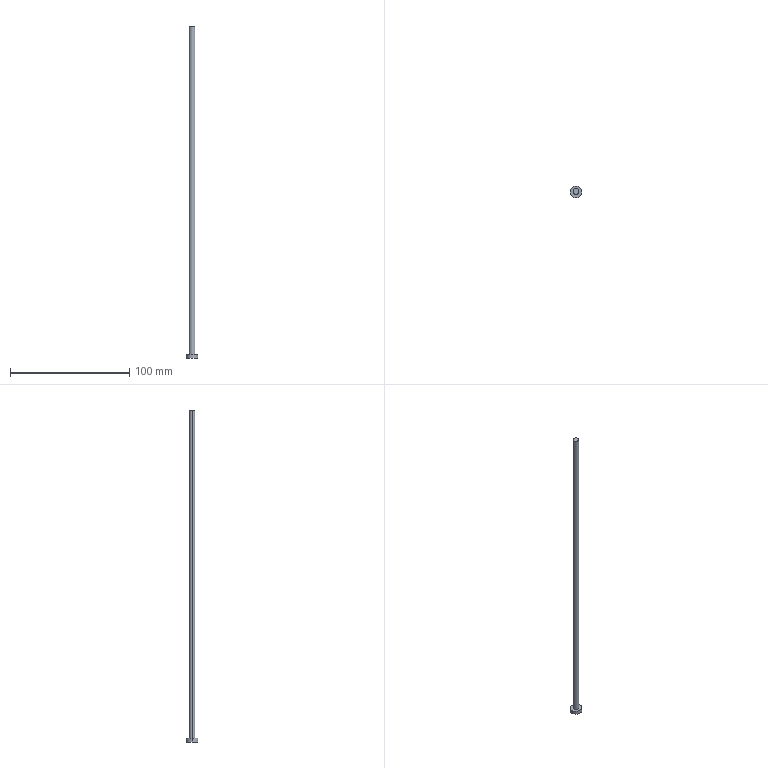Part | Creo | 1 solid | 7 faces | box 10 x 10 x 278.48 mm | volume 5645 mm3 | cylinder 4 | plane 3 | commonest cylinder face diameters 5 x2 10 x2
STEP:
#1=CARTESIAN_POINT('',(-182.5,235.,42.98));
#2=VERTEX_POINT('',#1);
#3=CARTESIAN_POINT('',(-187.5,235.,42.98));
#4=VERTEX_POINT('',#3);
#5=CARTESIAN_POINT('',(-185.,235.,42.98));
#6=DIRECTION('',(0.,0.,1.));
#7=DIRECTION('',(1.,0.,0.));
#8=AXIS2_PLACEMENT_3D('',#5,#6,#7);
#9=CIRCLE('',#8,2.5);
#10=EDGE_CURVE('',#2,#4,#9,.T.);
#11=ORIENTED_EDGE('',*,*,#10,.T.);
#12=CARTESIAN_POINT('',(-187.5,235.,-232.5));
#13=VERTEX_POINT('',#12);
#14=CARTESIAN_POINT('',(-187.5,235.,42.98));
#15=DIRECTION('',(0.,0.,-1.));
#16=VECTOR('',#15,275.48);
#17=LINE('',#14,#16);
#18=EDGE_CURVE('',#4,#13,#17,.T.);
#19=ORIENTED_EDGE('',*,*,#18,.T.);
#20=CARTESIAN_POINT('',(-182.5,235.,-232.5));
#21=VERTEX_POINT('',#20);
#22=CARTESIAN_POINT('',(-185.,235.,-232.5));
#23=DIRECTION('',(0.,0.,-1.));
#24=DIRECTION('',(-1.,0.,0.));
#25=AXIS2_PLACEMENT_3D('',#22,#23,#24);
#26=CIRCLE('',#25,2.5);
#27=EDGE_CURVE('',#13,#21,#26,.T.);
#28=ORIENTED_EDGE('',*,*,#27,.T.);
#29=CARTESIAN_POINT('',(-182.5,235.,42.98));
#30=DIRECTION('',(0.,0.,-1.));
#31=VECTOR('',#30,275.48);
#32=LINE('',#29,#31);
#33=EDGE_CURVE('',#2,#21,#32,.T.);
#34=ORIENTED_EDGE('',*,*,#33,.F.);
#35=EDGE_LOOP('',(#11,#19,#28,#34));
#36=FACE_OUTER_BOUND('',#35,.F.);
#37=CARTESIAN_POINT('',(-185.,235.,49.5));
#38=DIRECTION('',(0.,0.,-1.));
#39=DIRECTION('',(-1.,0.,0.));
#40=AXIS2_PLACEMENT_3D('',#37,#38,#39);
#41=CYLINDRICAL_SURFACE('',#40,2.5);
#42=ADVANCED_FACE('',(#36),#41,.T.);
#43=CARTESIAN_POINT('',(-185.,235.,42.98));
#44=DIRECTION('',(0.,0.,1.));
#45=DIRECTION('',(-1.,0.,0.));
#46=AXIS2_PLACEMENT_3D('',#43,#44,#45);
#47=CIRCLE('',#46,2.5);
#48=EDGE_CURVE('',#4,#2,#47,.T.);
#49=ORIENTED_EDGE('',*,*,#48,.F.);
#50=ORIENTED_EDGE('',*,*,#10,.F.);
#51=EDGE_LOOP('',(#49,#50));
#52=FACE_OUTER_BOUND('',#51,.F.);
#53=CARTESIAN_POINT('',(-179.214,-235.438,42.98));
#54=DIRECTION('',(0.,0.,-1.));
#55=DIRECTION('',(0.,1.,0.));
#56=AXIS2_PLACEMENT_3D('',#53,#54,#55);
#57=PLANE('',#56);
#58=ADVANCED_FACE('',(#52),#57,.F.);
#59=ORIENTED_EDGE('',*,*,#48,.T.);
#60=ORIENTED_EDGE('',*,*,#33,.T.);
#61=CARTESIAN_POINT('',(-185.,235.,-232.5));
#62=DIRECTION('',(0.,0.,-1.));
#63=DIRECTION('',(1.,0.,0.));
#64=AXIS2_PLACEMENT_3D('',#61,#62,#63);
#65=CIRCLE('',#64,2.5);
#66=EDGE_CURVE('',#21,#13,#65,.T.);
#67=ORIENTED_EDGE('',*,*,#66,.T.);
#68=ORIENTED_EDGE('',*,*,#18,.F.);
#69=EDGE_LOOP('',(#59,#60,#67,#68));
#70=FACE_OUTER_BOUND('',#69,.F.);
#71=CARTESIAN_POINT('',(-185.,235.,49.5));
#72=DIRECTION('',(0.,0.,-1.));
#73=DIRECTION('',(-1.,0.,0.));
#74=AXIS2_PLACEMENT_3D('',#71,#72,#73);
#75=CYLINDRICAL_SURFACE('',#74,2.5);
#76=ADVANCED_FACE('',(#70),#75,.T.);
#77=CARTESIAN_POINT('',(-190.,235.,-232.5));
#78=VERTEX_POINT('',#77);
#79=CARTESIAN_POINT('',(-180.,235.,-232.5));
#80=VERTEX_POINT('',#79);
#81=CARTESIAN_POINT('',(-185.,235.,-232.5));
#82=DIRECTION('',(0.,0.,1.));
#83=DIRECTION('',(-1.,0.,0.));
#84=AXIS2_PLACEMENT_3D('',#81,#82,#83);
#85=CIRCLE('',#84,5.);
#86=EDGE_CURVE('',#78,#80,#85,.T.);
#87=ORIENTED_EDGE('',*,*,#86,.F.);
#88=CARTESIAN_POINT('',(-185.,235.,-232.5));
#89=DIRECTION('',(0.,0.,1.));
#90=DIRECTION('',(1.,0.,0.));
#91=AXIS2_PLACEMENT_3D('',#88,#89,#90);
#92=CIRCLE('',#91,5.);
#93=EDGE_CURVE('',#80,#78,#92,.T.);
#94=ORIENTED_EDGE('',*,*,#93,.F.);
#95=EDGE_LOOP('',(#87,#94));
#96=FACE_OUTER_BOUND('',#95,.F.);
#97=ORIENTED_EDGE('',*,*,#27,.F.);
#98=ORIENTED_EDGE('',*,*,#66,.F.);
#99=EDGE_LOOP('',(#97,#98));
#100=FACE_BOUND('',#99,.F.);
#101=CARTESIAN_POINT('',(-185.,235.,-232.5));
#102=DIRECTION('',(0.,0.,-1.));
#103=DIRECTION('',(-1.,0.,0.));
#104=AXIS2_PLACEMENT_3D('',#101,#102,#103);
#105=PLANE('',#104);
#106=ADVANCED_FACE('',(#96,#100),#105,.F.);
#107=CARTESIAN_POINT('',(-180.,235.,-235.5));
#108=VERTEX_POINT('',#107);
#109=CARTESIAN_POINT('',(-190.,235.,-235.5));
#110=VERTEX_POINT('',#109);
#111=CARTESIAN_POINT('',(-185.,235.,-235.5));
#112=DIRECTION('',(0.,0.,-1.));
#113=DIRECTION('',(1.,0.,0.));
#114=AXIS2_PLACEMENT_3D('',#111,#112,#113);
#115=CIRCLE('',#114,5.);
#116=EDGE_CURVE('',#108,#110,#115,.T.);
#117=ORIENTED_EDGE('',*,*,#116,.T.);
#118=CARTESIAN_POINT('',(-190.,235.,-232.5));
#119=DIRECTION('',(0.,0.,-1.));
#120=VECTOR('',#119,3.);
#121=LINE('',#118,#120);
#122=EDGE_CURVE('',#78,#110,#121,.T.);
#123=ORIENTED_EDGE('',*,*,#122,.F.);
#124=ORIENTED_EDGE('',*,*,#86,.T.);
#125=CARTESIAN_POINT('',(-180.,235.,-232.5));
#126=DIRECTION('',(0.,0.,-1.));
#127=VECTOR('',#126,3.);
#128=LINE('',#125,#127);
#129=EDGE_CURVE('',#80,#108,#128,.T.);
#130=ORIENTED_EDGE('',*,*,#129,.T.);
#131=EDGE_LOOP('',(#117,#123,#124,#130));
#132=FACE_OUTER_BOUND('',#131,.F.);
#133=CARTESIAN_POINT('',(-185.,235.,-245.913));
#134=DIRECTION('',(0.,0.,-1.));
#135=DIRECTION('',(-1.,0.,0.));
#136=AXIS2_PLACEMENT_3D('',#133,#134,#135);
#137=CYLINDRICAL_SURFACE('',#136,5.);
#138=ADVANCED_FACE('',(#132),#137,.T.);
#139=ORIENTED_EDGE('',*,*,#116,.F.);
#140=CARTESIAN_POINT('',(-185.,235.,-235.5));
#141=DIRECTION('',(0.,0.,-1.));
#142=DIRECTION('',(-1.,0.,0.));
#143=AXIS2_PLACEMENT_3D('',#140,#141,#142);
#144=CIRCLE('',#143,5.);
#145=EDGE_CURVE('',#110,#108,#144,.T.);
#146=ORIENTED_EDGE('',*,*,#145,.F.);
#147=EDGE_LOOP('',(#139,#146));
#148=FACE_OUTER_BOUND('',#147,.F.);
#149=CARTESIAN_POINT('',(-181.,235.,-235.5));
#150=DIRECTION('',(0.,0.,1.));
#151=DIRECTION('',(1.,0.,0.));
#152=AXIS2_PLACEMENT_3D('',#149,#150,#151);
#153=PLANE('',#152);
#154=ADVANCED_FACE('',(#148),#153,.F.);
#155=ORIENTED_EDGE('',*,*,#145,.T.);
#156=ORIENTED_EDGE('',*,*,#129,.F.);
#157=ORIENTED_EDGE('',*,*,#93,.T.);
#158=ORIENTED_EDGE('',*,*,#122,.T.);
#159=EDGE_LOOP('',(#155,#156,#157,#158));
#160=FACE_OUTER_BOUND('',#159,.F.);
#161=CARTESIAN_POINT('',(-185.,235.,-245.913));
#162=DIRECTION('',(0.,0.,-1.));
#163=DIRECTION('',(-1.,0.,0.));
#164=AXIS2_PLACEMENT_3D('',#161,#162,#163);
#165=CYLINDRICAL_SURFACE('',#164,5.);
#166=ADVANCED_FACE('',(#160),#165,.T.);
#167=CLOSED_SHELL('',(#42,#58,#76,#106,#138,#154,#166));
#168=MANIFOLD_SOLID_BREP('',#167);
#169=(LENGTH_UNIT()NAMED_UNIT(*)SI_UNIT(.MILLI.,.METRE.));
#170=UNCERTAINTY_MEASURE_WITH_UNIT(LENGTH_MEASURE(0.02788),#169,'','');
#171=(NAMED_UNIT(*)PLANE_ANGLE_UNIT()SI_UNIT($,.RADIAN.));
#172=PLANE_ANGLE_MEASURE_WITH_UNIT(PLANE_ANGLE_MEASURE(0.01745),#171);
#173=(CONVERSION_BASED_UNIT('DEGREE',#172)NAMED_UNIT(*)PLANE_ANGLE_UNIT());
#174=(NAMED_UNIT(*)SI_UNIT($,.STERADIAN.)SOLID_ANGLE_UNIT());
#175=(GEOMETRIC_REPRESENTATION_CONTEXT(3)GLOBAL_UNCERTAINTY_ASSIGNED_CONTEXT((#170))GLOBAL_UNIT_ASSIGNED_CONTEXT((#169,#173,#174))REPRESENTATION_CONTEXT('',''));
#176=ADVANCED_BREP_SHAPE_REPRESENTATION('',(#168),#175);